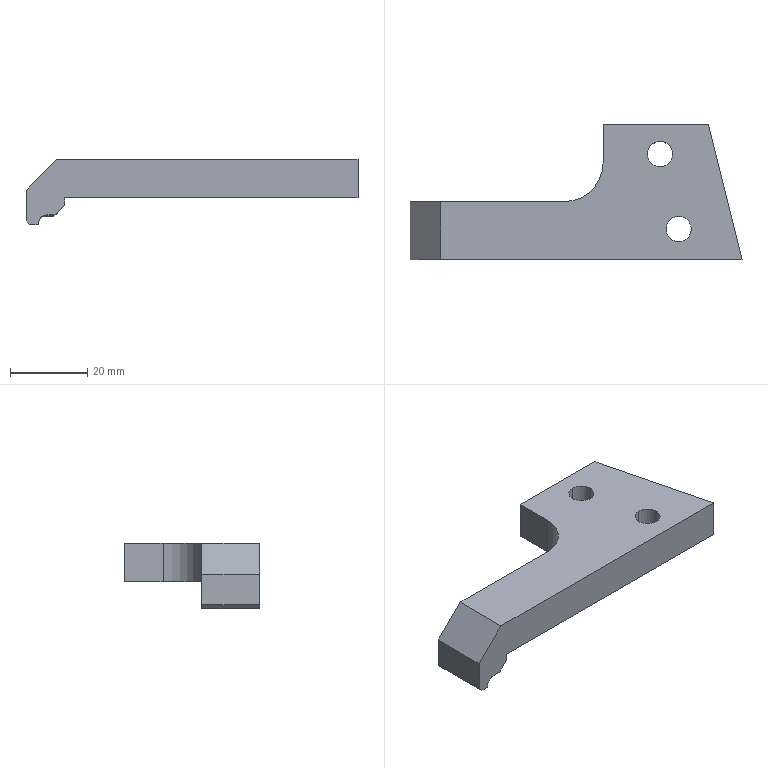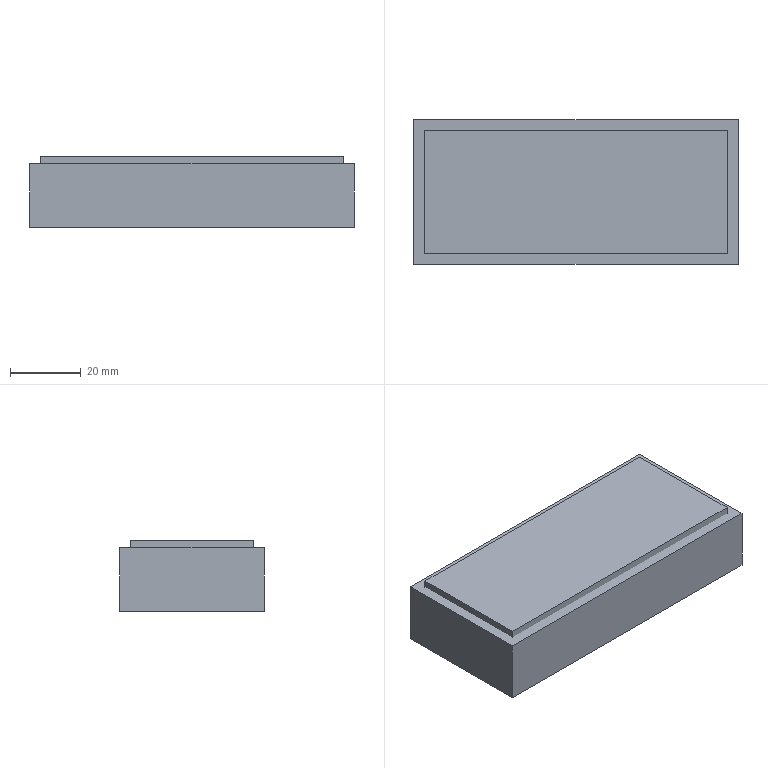CAM job | NX | 3-axis milling, drilling | part box 86 x 35 x 17 mm | stock box 92 x 41 x 20 mm
Tools:
number,name,description,diameter,corner_radius,flute_length,length,flutes
1,D63,Milling Tool-5 Parameters,63.0,0.0,50.0,75.0,2
10,D10,Milling Tool-5 Parameters,10.0,0.0,50.0,75.0,2
11,D10JING,Milling Tool-5 Parameters,10.0,0.0,50.0,75.0,2
7,D6A45,Milling Tool-5 Parameters,6.0,0.0,3.0,3.0,2
14,6.5ZT,Drilling Tool,4.8,0.0,35.0,50.0,2
5,D6R0.5,Milling Tool-5 Parameters,6.0,0.5,50.0,75.0,2
Operations:
program,operation,operation_type,tool,method,geometry_group,spindle_rpm,surface_speed,feed_per_tooth,feed_cut,feed_plunge,cut_length_mm,path_length_mm,cut_time_min,machine_time_min
1-90-40-20毛胚,FLOOR_WALL,VolumeBased25DMillingOperation,D63,METHOD,A,6500.0,1286.0,0.0962,1250.0,100.0,167.0,221.0,0.1336,0.139
1-90-40-20毛胚,ADAPTIVE_MILLING,CavityMilling,D10,METHOD,A,9500.0,298.0,0.1579,3000.0,1000.0,4862.328,5601.988,1.626,1.7
1-90-40-20毛胚,ZLEVEL_PROFILE_COPY_COPY_1_COPY,ZLevelMilling,D10JING,METHOD,A,9500.0,298.0,0.0632,1200.0,100.0,269.49,357.49,0.2246,0.2334
1-90-40-20毛胚,DRILLING_COPY_1,Operation,D6A45,METHOD,A,5000.0,94.0,0.025,250.0,0.0,8.0,99.224,0.032,0.0411
1-90-40-20毛胚,DRILLING_COPY_COPY_1,Operation,6.5ZT,METHOD,A,2000.0,15.0,0.03,120.0,0.0,31.884,146.992,0.2657,0.2772
1-90-40-20毛胚,ZLEVEL_PROFILE_COPY_1_COPY_1_COPY_1_1,ZLevelMilling,D6R0.5,METHOD,A,9500.0,119.0,0.1053,2000.0,800.0,1934.129,1999.643,0.9693,0.9759
1-90-40-20毛胚,ZLEVEL_PROFILE_1_COPY_1_COPY_COPY_1,ZLevelMilling,D6A45,METHOD,A,9500.0,179.0,0.0526,1000.0,100.0,246.097,506.683,0.2461,0.2722
2-90-40-20毛胚,FLOOR_WALL_COPY,VolumeBased25DMillingOperation,D63,METHOD,B,6500.0,1286.0,0.0962,1250.0,100.0,483.0,949.001,0.3864,0.433
2-90-40-20毛胚,FLOOR_WALL_1,VolumeBased25DMillingOperation,D10,METHOD,B,9500.0,298.0,0.1158,2200.0,1000.0,2901.796,3079.247,1.355,1.373
2-90-40-20毛胚,FLOOR_WALL_1_1,VolumeBased25DMillingOperation,D10JING,METHOD,B,9500.0,179.0,0.0658,1250.0,100.0,671.9,841.905,0.5375,0.5545
2-90-40-20毛胚,FIXED_CONTOUR_COPY,SurfaceContour,D6R0.5,METHOD,B,9500.0,89.0,0.1053,2000.0,1000.0,1048.526,1107.111,0.5267,0.5325
2-90-40-20毛胚,FIXED_CONTOUR,SurfaceContour,D6R0.5,METHOD,B,9500.0,89.0,0.1053,2000.0,1000.0,1704.546,1753.746,0.8562,0.8611
2-90-40-20毛胚,ZLEVEL_PROFILE_COPY_1_COPY_1_COPY_1_1_COPY_COPY,ZLevelMilling,D6R0.5,METHOD,B,9500.0,119.0,0.1053,2000.0,800.0,342.231,400.745,0.1734,0.1792
2-90-40-20毛胚,ZLEVEL_PROFILE_1_COPY_1_COPY_COPY_1_COPY,ZLevelMilling,D6A45,METHOD,B,9500.0,179.0,0.0526,1000.0,100.0,236.186,540.068,0.2362,0.2666